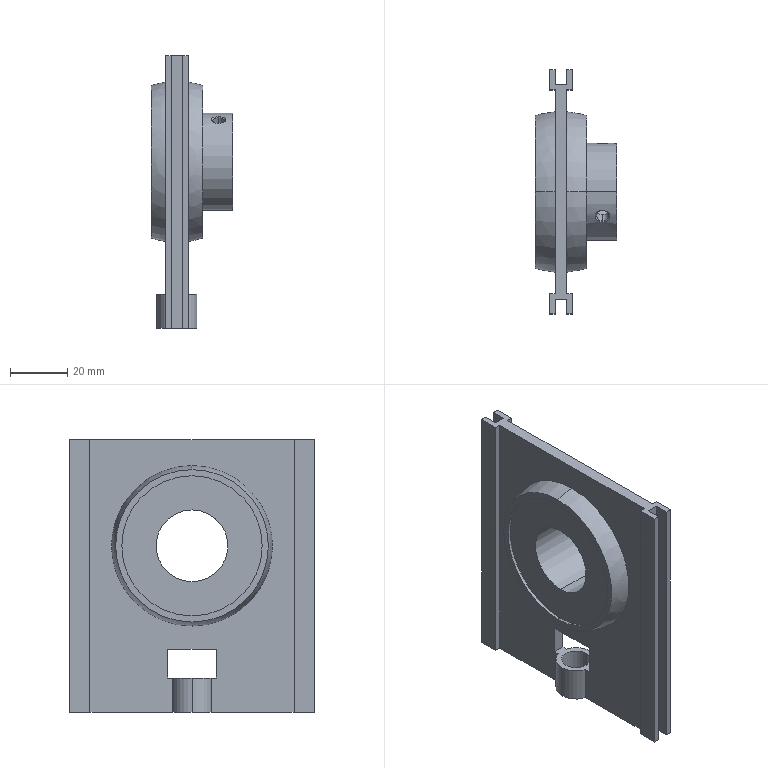Part | STEP file | _TUUFLN25_BE.stp | 1 solid | 56 faces | box 28.5 x 85 x 95 mm | volume 58062 mm3 | plane 31 | cylinder 13 | sphere 8 | cone 4 | commonest cylinder face diameters 4.134 x4 14 x3 10 x2 25 x2 33.9 x2